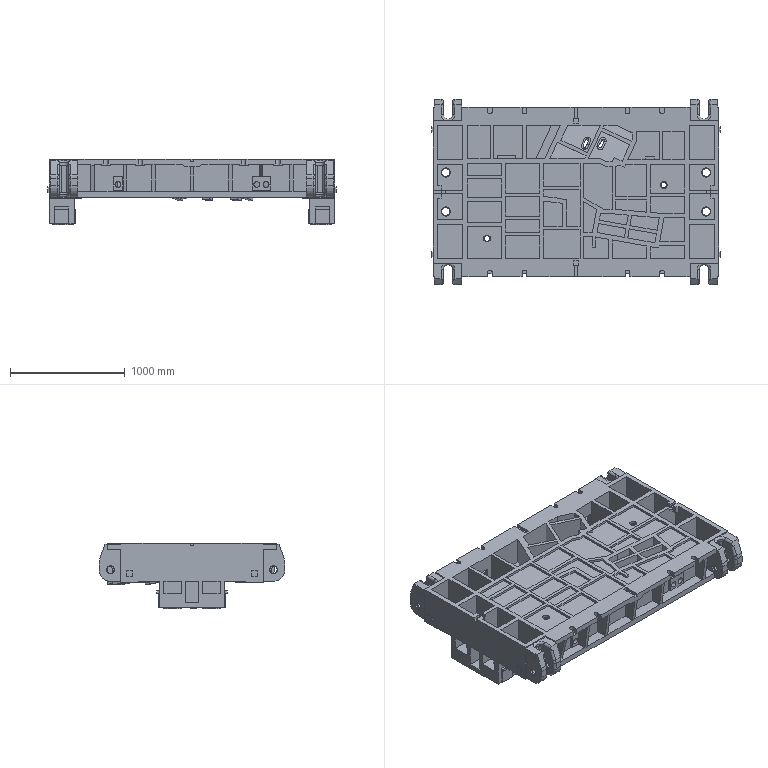Part | NX | features solid 2 | 1 solid | 1620 faces | box 2510 x 1620 x 570 mm | volume 479376372 mm3 | plane 1367 | cylinder 223 | torus 24 | spline 6 | commonest cylinder face diameters 40 x48 68 x48 80 x24 70 x18 64 x16 200 x16